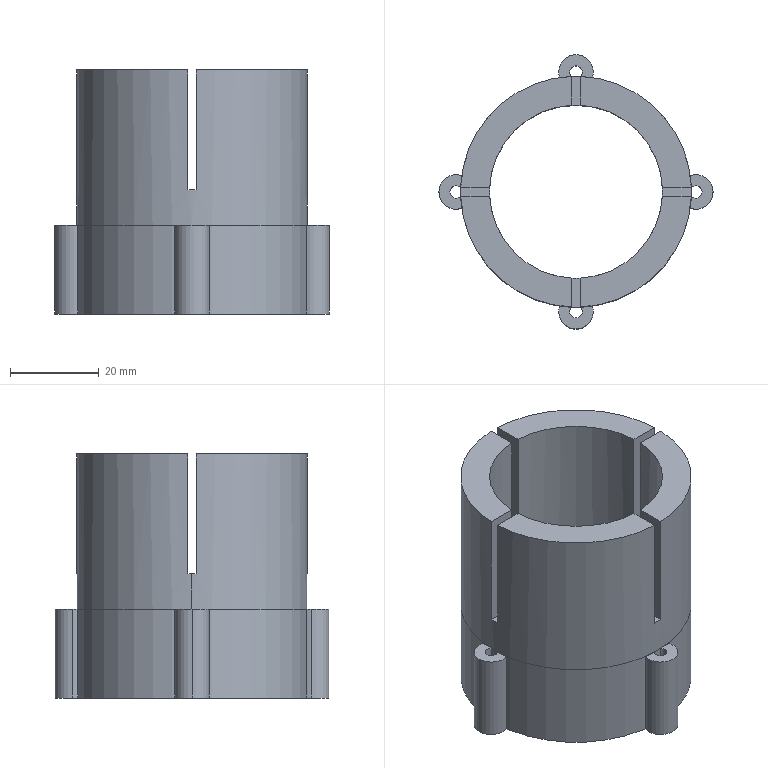Part | SolidWorks | 6 solids | 353 faces | box 61.8 x 61.8 x 55 mm | volume 44978 mm3 | plane 223 | spline 98 | cylinder 32 | commonest cylinder face diameters 52 x12 2.8 x9 7.8 x9 39 x2